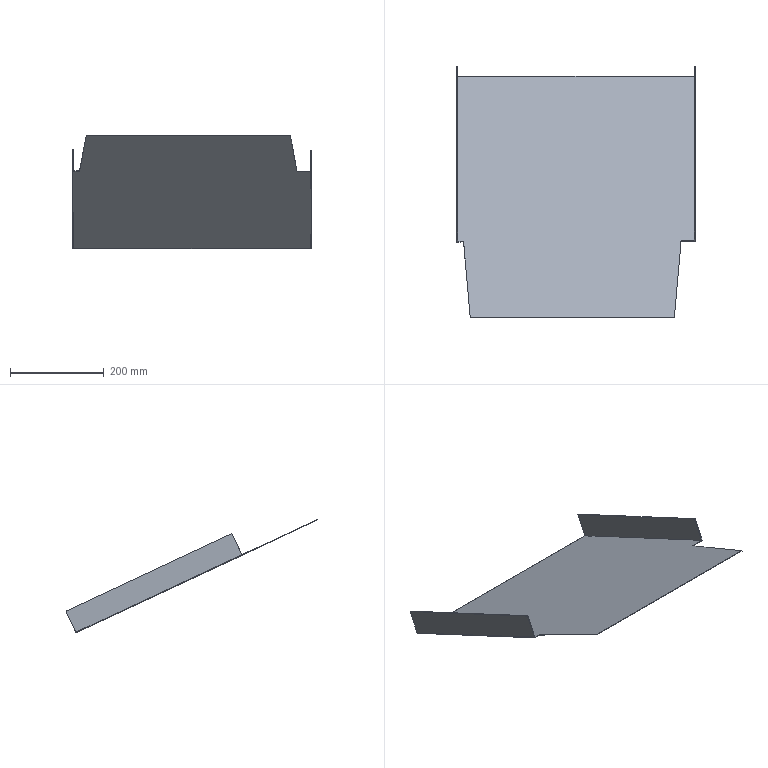Part | NX | features solid 2 | 1 solid | 17 faces | box 510 x 538.761 x 242.084 mm | volume 358465 mm3 | plane 15 | spline 2
STEP:
#1=CARTESIAN_POINT('',(348.,1102.315,-269.141));
#2=VERTEX_POINT('',#1);
#3=CARTESIAN_POINT('',(-158.,1102.315,-269.141));
#4=VERTEX_POINT('',#3);
#5=CARTESIAN_POINT('',(-1100.,1102.315,-269.141));
#6=DIRECTION('',(1.,0.,0.));
#7=VECTOR('',#6,1000.);
#8=LINE('',#5,#7);
#9=EDGE_CURVE('',#2,#4,#8,.F.);
#10=ORIENTED_EDGE('',*,*,#9,.T.);
#11=CARTESIAN_POINT('',(-158.,747.462,-103.67));
#12=VERTEX_POINT('',#11);
#13=CARTESIAN_POINT('',(-158.,630.423,-49.094));
#14=DIRECTION('',(0.,0.9063,-0.4226));
#15=VECTOR('',#14,1000.);
#16=LINE('',#13,#15);
#17=EDGE_CURVE('',#4,#12,#16,.F.);
#18=ORIENTED_EDGE('',*,*,#17,.T.);
#19=CARTESIAN_POINT('',(-145.428,747.563,-103.717));
#20=VERTEX_POINT('',#19);
#21=CARTESIAN_POINT('',(-145.428,747.563,-103.717));
#22=CARTESIAN_POINT('',(-148.187,747.54,-103.707));
#23=CARTESIAN_POINT('',(-152.378,747.509,-103.692));
#24=CARTESIAN_POINT('',(-158.,747.469,-103.673));
#25=B_SPLINE_CURVE_WITH_KNOTS('',3,(#21,#22,#23,#24),.UNSPECIFIED.,.F.,.F.,(4,4),(0.,0.1284),.UNSPECIFIED.);
#26=EDGE_CURVE('',#12,#20,#25,.F.);
#27=ORIENTED_EDGE('',*,*,#26,.T.);
#28=CARTESIAN_POINT('',(-131.215,585.107,-27.963));
#29=VERTEX_POINT('',#28);
#30=CARTESIAN_POINT('',(-37.805,-482.577,469.906));
#31=DIRECTION('',(0.07904,-0.9035,0.4213));
#32=VECTOR('',#31,1000.);
#33=LINE('',#30,#32);
#34=EDGE_CURVE('',#29,#20,#33,.F.);
#35=ORIENTED_EDGE('',*,*,#34,.F.);
#36=CARTESIAN_POINT('',(305.318,585.107,-27.963));
#37=VERTEX_POINT('',#36);
#38=CARTESIAN_POINT('',(-1100.,585.107,-27.963));
#39=DIRECTION('',(-1.,0.,0.));
#40=VECTOR('',#39,1000.);
#41=LINE('',#38,#40);
#42=EDGE_CURVE('',#29,#37,#41,.F.);
#43=ORIENTED_EDGE('',*,*,#42,.T.);
#44=CARTESIAN_POINT('',(319.689,749.371,-104.56));
#45=VERTEX_POINT('',#44);
#46=CARTESIAN_POINT('',(300.478,529.781,-2.164));
#47=DIRECTION('',(0.07904,0.9035,-0.4213));
#48=VECTOR('',#47,1000.);
#49=LINE('',#46,#48);
#50=EDGE_CURVE('',#45,#37,#49,.F.);
#51=ORIENTED_EDGE('',*,*,#50,.F.);
#52=CARTESIAN_POINT('',(348.,749.432,-104.589));
#53=VERTEX_POINT('',#52);
#54=CARTESIAN_POINT('',(348.,749.428,-104.587));
#55=CARTESIAN_POINT('',(338.843,749.394,-104.571));
#56=CARTESIAN_POINT('',(329.406,749.375,-104.562));
#57=CARTESIAN_POINT('',(319.689,749.371,-104.56));
#58=B_SPLINE_CURVE_WITH_KNOTS('',3,(#54,#55,#56,#57),.UNSPECIFIED.,.F.,.F.,(4,4),(0.8994,1.),.UNSPECIFIED.);
#59=EDGE_CURVE('',#53,#45,#58,.T.);
#60=ORIENTED_EDGE('',*,*,#59,.F.);
#61=CARTESIAN_POINT('',(348.,630.423,-49.094));
#62=DIRECTION('',(0.,0.9063,-0.4226));
#63=VECTOR('',#62,1000.);
#64=LINE('',#61,#63);
#65=EDGE_CURVE('',#2,#53,#64,.F.);
#66=ORIENTED_EDGE('',*,*,#65,.F.);
#67=EDGE_LOOP('',(#10,#18,#27,#35,#43,#51,#60,#66));
#68=FACE_BOUND('',#67,.T.);
#69=CARTESIAN_POINT('',(-1100.,630.423,-49.094));
#70=DIRECTION('',(0.,-0.4226,-0.9063));
#71=DIRECTION('',(0.,-0.9063,0.4226));
#72=AXIS2_PLACEMENT_3D('',#69,#70,#71);
#73=PLANE('',#72);
#74=ADVANCED_FACE('',(#68),#73,.F.);
#75=CARTESIAN_POINT('',(350.,1101.892,-270.047));
#76=VERTEX_POINT('',#75);
#77=CARTESIAN_POINT('',(-160.,1101.892,-270.047));
#78=VERTEX_POINT('',#77);
#79=CARTESIAN_POINT('',(-1100.,1101.892,-270.047));
#80=DIRECTION('',(1.,0.,0.));
#81=VECTOR('',#80,1000.);
#82=LINE('',#79,#81);
#83=EDGE_CURVE('',#76,#78,#82,.F.);
#84=ORIENTED_EDGE('',*,*,#83,.F.);
#85=CARTESIAN_POINT('',(350.,749.013,-105.497));
#86=VERTEX_POINT('',#85);
#87=CARTESIAN_POINT('',(350.,630.,-50.));
#88=DIRECTION('',(0.,0.9063,-0.4226));
#89=VECTOR('',#88,1000.);
#90=LINE('',#87,#89);
#91=EDGE_CURVE('',#76,#86,#90,.F.);
#92=ORIENTED_EDGE('',*,*,#91,.T.);
#93=CARTESIAN_POINT('',(319.689,748.949,-105.467));
#94=VERTEX_POINT('',#93);
#95=CARTESIAN_POINT('',(350.,749.013,-105.497));
#96=CARTESIAN_POINT('',(340.219,748.974,-105.478));
#97=CARTESIAN_POINT('',(330.116,748.953,-105.468));
#98=CARTESIAN_POINT('',(319.689,748.949,-105.467));
#99=B_SPLINE_CURVE_WITH_KNOTS('',3,(#95,#96,#97,#98),.UNSPECIFIED.,.F.,.F.,(4,4),(0.8921,1.),.UNSPECIFIED.);
#100=EDGE_CURVE('',#86,#94,#99,.T.);
#101=ORIENTED_EDGE('',*,*,#100,.T.);
#102=CARTESIAN_POINT('',(305.318,584.685,-28.869));
#103=VERTEX_POINT('',#102);
#104=CARTESIAN_POINT('',(300.478,529.358,-3.07));
#105=DIRECTION('',(0.07904,0.9035,-0.4213));
#106=VECTOR('',#105,1000.);
#107=LINE('',#104,#106);
#108=EDGE_CURVE('',#94,#103,#107,.F.);
#109=ORIENTED_EDGE('',*,*,#108,.T.);
#110=CARTESIAN_POINT('',(-131.215,584.685,-28.869));
#111=VERTEX_POINT('',#110);
#112=CARTESIAN_POINT('',(-1100.,584.685,-28.869));
#113=DIRECTION('',(-1.,0.,0.));
#114=VECTOR('',#113,1000.);
#115=LINE('',#112,#114);
#116=EDGE_CURVE('',#111,#103,#115,.F.);
#117=ORIENTED_EDGE('',*,*,#116,.F.);
#118=CARTESIAN_POINT('',(-145.428,747.141,-104.624));
#119=VERTEX_POINT('',#118);
#120=CARTESIAN_POINT('',(-37.805,-482.999,469.));
#121=DIRECTION('',(0.07904,-0.9035,0.4213));
#122=VECTOR('',#121,1000.);
#123=LINE('',#120,#122);
#124=EDGE_CURVE('',#111,#119,#123,.F.);
#125=ORIENTED_EDGE('',*,*,#124,.T.);
#126=CARTESIAN_POINT('',(-158.,747.043,-104.578));
#127=VERTEX_POINT('',#126);
#128=CARTESIAN_POINT('',(-145.428,747.141,-104.624));
#129=CARTESIAN_POINT('',(-148.187,747.118,-104.613));
#130=CARTESIAN_POINT('',(-152.378,747.087,-104.598));
#131=CARTESIAN_POINT('',(-158.,747.047,-104.58));
#132=B_SPLINE_CURVE_WITH_KNOTS('',3,(#128,#129,#130,#131),.UNSPECIFIED.,.F.,.F.,(4,4),(0.,0.1284),.UNSPECIFIED.);
#133=EDGE_CURVE('',#127,#119,#132,.F.);
#134=ORIENTED_EDGE('',*,*,#133,.F.);
#135=CARTESIAN_POINT('',(-160.,747.032,-104.573));
#136=VERTEX_POINT('',#135);
#137=CARTESIAN_POINT('',(-158.,747.047,-104.58));
#138=CARTESIAN_POINT('',(-158.648,747.042,-104.578));
#139=CARTESIAN_POINT('',(-159.314,747.037,-104.575));
#140=CARTESIAN_POINT('',(-160.,747.032,-104.573));
#141=B_SPLINE_CURVE_WITH_KNOTS('',3,(#137,#138,#139,#140),.UNSPECIFIED.,.F.,.F.,(4,4),(0.1284,0.1432),.UNSPECIFIED.);
#142=EDGE_CURVE('',#127,#136,#141,.T.);
#143=ORIENTED_EDGE('',*,*,#142,.T.);
#144=CARTESIAN_POINT('',(-160.,630.,-50.));
#145=DIRECTION('',(0.,0.9063,-0.4226));
#146=VECTOR('',#145,1000.);
#147=LINE('',#144,#146);
#148=EDGE_CURVE('',#78,#136,#147,.F.);
#149=ORIENTED_EDGE('',*,*,#148,.F.);
#150=EDGE_LOOP('',(#84,#92,#101,#109,#117,#125,#134,#143,#149));
#151=FACE_BOUND('',#150,.T.);
#152=CARTESIAN_POINT('',(-1100.,630.,-50.));
#153=DIRECTION('',(0.,-0.4226,-0.9063));
#154=DIRECTION('',(0.,-0.9063,0.4226));
#155=AXIS2_PLACEMENT_3D('',#152,#153,#154);
#156=PLANE('',#155);
#157=ADVANCED_FACE('',(#151),#156,.T.);
#158=CARTESIAN_POINT('',(350.,1123.446,-223.825));
#159=VERTEX_POINT('',#158);
#160=CARTESIAN_POINT('',(350.,1101.892,-270.047));
#161=DIRECTION('',(0.,-0.4226,-0.9063));
#162=VECTOR('',#161,1000.);
#163=LINE('',#160,#162);
#164=EDGE_CURVE('',#159,#76,#163,.T.);
#165=ORIENTED_EDGE('',*,*,#164,.T.);
#166=ORIENTED_EDGE('',*,*,#83,.T.);
#167=CARTESIAN_POINT('',(-160.,1123.446,-223.825));
#168=VERTEX_POINT('',#167);
#169=CARTESIAN_POINT('',(-160.,1101.892,-270.047));
#170=DIRECTION('',(0.,-0.4226,-0.9063));
#171=VECTOR('',#170,1000.);
#172=LINE('',#169,#171);
#173=EDGE_CURVE('',#168,#78,#172,.T.);
#174=ORIENTED_EDGE('',*,*,#173,.F.);
#175=CARTESIAN_POINT('',(-158.,1123.446,-223.825));
#176=VERTEX_POINT('',#175);
#177=CARTESIAN_POINT('',(-160.,1123.446,-223.825));
#178=DIRECTION('',(1.,0.,0.));
#179=VECTOR('',#178,1000.);
#180=LINE('',#177,#179);
#181=EDGE_CURVE('',#176,#168,#180,.F.);
#182=ORIENTED_EDGE('',*,*,#181,.F.);
#183=CARTESIAN_POINT('',(-158.,1101.892,-270.047));
#184=DIRECTION('',(0.,0.4226,0.9063));
#185=VECTOR('',#184,1000.);
#186=LINE('',#183,#185);
#187=EDGE_CURVE('',#4,#176,#186,.T.);
#188=ORIENTED_EDGE('',*,*,#187,.F.);
#189=ORIENTED_EDGE('',*,*,#9,.F.);
#190=CARTESIAN_POINT('',(348.,1123.446,-223.825));
#191=VERTEX_POINT('',#190);
#192=CARTESIAN_POINT('',(348.,1101.892,-270.047));
#193=DIRECTION('',(0.,0.4226,0.9063));
#194=VECTOR('',#193,1000.);
#195=LINE('',#192,#194);
#196=EDGE_CURVE('',#2,#191,#195,.T.);
#197=ORIENTED_EDGE('',*,*,#196,.T.);
#198=CARTESIAN_POINT('',(350.,1123.446,-223.825));
#199=DIRECTION('',(1.,0.,0.));
#200=VECTOR('',#199,1000.);
#201=LINE('',#198,#200);
#202=EDGE_CURVE('',#191,#159,#201,.T.);
#203=ORIENTED_EDGE('',*,*,#202,.T.);
#204=EDGE_LOOP('',(#165,#166,#174,#182,#188,#189,#197,#203));
#205=FACE_BOUND('',#204,.T.);
#206=CARTESIAN_POINT('',(-1100.,1101.892,-270.047));
#207=DIRECTION('',(0.,-0.9063,0.4226));
#208=DIRECTION('',(0.,0.4226,0.9063));
#209=AXIS2_PLACEMENT_3D('',#206,#207,#208);
#210=PLANE('',#209);
#211=ADVANCED_FACE('',(#205),#210,.F.);
#212=CARTESIAN_POINT('',(350.,749.436,-104.59));
#213=VERTEX_POINT('',#212);
#214=CARTESIAN_POINT('',(350.,749.436,-104.59));
#215=CARTESIAN_POINT('',(349.333,749.436,-104.59));
#216=CARTESIAN_POINT('',(348.667,749.436,-104.59));
#217=CARTESIAN_POINT('',(348.,749.436,-104.59));
#218=B_SPLINE_CURVE_WITH_KNOTS('',3,(#214,#215,#216,#217),.UNSPECIFIED.,.F.,.F.,(4,4),(0.,1.),.UNSPECIFIED.);
#219=EDGE_CURVE('',#213,#53,#218,.T.);
#220=ORIENTED_EDGE('',*,*,#219,.T.);
#221=ORIENTED_EDGE('',*,*,#59,.T.);
#222=CARTESIAN_POINT('',(319.689,748.949,-105.467));
#223=CARTESIAN_POINT('',(319.689,749.09,-105.165));
#224=CARTESIAN_POINT('',(319.689,749.23,-104.862));
#225=CARTESIAN_POINT('',(319.689,749.371,-104.56));
#226=B_SPLINE_CURVE_WITH_KNOTS('',3,(#222,#223,#224,#225),.UNSPECIFIED.,.F.,.F.,(4,4),(0.,1.),.UNSPECIFIED.);
#227=EDGE_CURVE('',#94,#45,#226,.T.);
#228=ORIENTED_EDGE('',*,*,#227,.F.);
#229=ORIENTED_EDGE('',*,*,#100,.F.);
#230=CARTESIAN_POINT('',(350.,749.013,-105.497));
#231=DIRECTION('',(0.,0.4226,0.9063));
#232=VECTOR('',#231,1000.);
#233=LINE('',#230,#232);
#234=EDGE_CURVE('',#213,#86,#233,.F.);
#235=ORIENTED_EDGE('',*,*,#234,.F.);
#236=EDGE_LOOP('',(#220,#221,#228,#229,#235));
#237=FACE_BOUND('',#236,.T.);
#238=CARTESIAN_POINT('',(350.,749.013,-105.497));
#239=CARTESIAN_POINT('',(350.,749.436,-104.59));
#240=CARTESIAN_POINT('',(340.219,748.974,-105.478));
#241=CARTESIAN_POINT('',(340.219,749.397,-104.572));
#242=CARTESIAN_POINT('',(330.116,748.953,-105.468));
#243=CARTESIAN_POINT('',(330.116,749.375,-104.562));
#244=CARTESIAN_POINT('',(319.689,748.949,-105.467));
#245=CARTESIAN_POINT('',(319.689,749.371,-104.56));
#246=B_SPLINE_SURFACE_WITH_KNOTS('',3,1,((#238,#239),(#240,#241),(#242,#243),(#244,#245)),.SURF_OF_LINEAR_EXTRUSION.,.F.,.F.,.F.,(4,4),(2,2),(0.8921,1.),(0.,1.),.PIECEWISE_BEZIER_KNOTS.);
#247=ADVANCED_FACE('',(#237),#246,.F.);
#248=ORIENTED_EDGE('',*,*,#133,.T.);
#249=CARTESIAN_POINT('',(-145.428,747.563,-103.717));
#250=CARTESIAN_POINT('',(-145.428,747.422,-104.019));
#251=CARTESIAN_POINT('',(-145.428,747.281,-104.321));
#252=CARTESIAN_POINT('',(-145.428,747.141,-104.624));
#253=B_SPLINE_CURVE_WITH_KNOTS('',3,(#249,#250,#251,#252),.UNSPECIFIED.,.F.,.F.,(4,4),(0.,1.),.UNSPECIFIED.);
#254=EDGE_CURVE('',#119,#20,#253,.F.);
#255=ORIENTED_EDGE('',*,*,#254,.T.);
#256=ORIENTED_EDGE('',*,*,#26,.F.);
#257=CARTESIAN_POINT('',(-158.,747.047,-104.58));
#258=DIRECTION('',(0.,0.4226,0.9063));
#259=VECTOR('',#258,1000.);
#260=LINE('',#257,#259);
#261=EDGE_CURVE('',#127,#12,#260,.T.);
#262=ORIENTED_EDGE('',*,*,#261,.F.);
#263=EDGE_LOOP('',(#248,#255,#256,#262));
#264=FACE_BOUND('',#263,.T.);
#265=CARTESIAN_POINT('',(-145.428,747.141,-104.624));
#266=CARTESIAN_POINT('',(-145.428,747.563,-103.717));
#267=CARTESIAN_POINT('',(-148.204,747.118,-104.613));
#268=CARTESIAN_POINT('',(-148.204,747.54,-103.707));
#269=CARTESIAN_POINT('',(-152.428,747.086,-104.598));
#270=CARTESIAN_POINT('',(-152.428,747.509,-103.692));
#271=CARTESIAN_POINT('',(-158.101,747.046,-104.579));
#272=CARTESIAN_POINT('',(-158.101,747.469,-103.673));
#273=B_SPLINE_SURFACE_WITH_KNOTS('',3,1,((#265,#266),(#267,#268),(#269,#270),(#271,#272)),.SURF_OF_LINEAR_EXTRUSION.,.F.,.F.,.F.,(4,4),(2,2),(0.,0.1292),(0.,1.),.PIECEWISE_BEZIER_KNOTS.);
#274=ADVANCED_FACE('',(#264),#273,.F.);
#275=ORIENTED_EDGE('',*,*,#34,.T.);
#276=ORIENTED_EDGE('',*,*,#254,.F.);
#277=ORIENTED_EDGE('',*,*,#124,.F.);
#278=CARTESIAN_POINT('',(-131.215,584.685,-28.869));
#279=DIRECTION('',(0.,0.4226,0.9063));
#280=VECTOR('',#279,1000.);
#281=LINE('',#278,#280);
#282=EDGE_CURVE('',#111,#29,#281,.T.);
#283=ORIENTED_EDGE('',*,*,#282,.T.);
#284=EDGE_LOOP('',(#275,#276,#277,#283));
#285=FACE_BOUND('',#284,.T.);
#286=CARTESIAN_POINT('',(-37.805,-482.999,469.));
#287=DIRECTION('',(-0.9969,-0.07164,0.03341));
#288=DIRECTION('',(-0.07168,0.9974,0.));
#289=AXIS2_PLACEMENT_3D('',#286,#287,#288);
#290=PLANE('',#289);
#291=ADVANCED_FACE('',(#285),#290,.T.);
#292=ORIENTED_EDGE('',*,*,#42,.F.);
#293=ORIENTED_EDGE('',*,*,#282,.F.);
#294=ORIENTED_EDGE('',*,*,#116,.T.);
#295=CARTESIAN_POINT('',(305.318,584.685,-28.869));
#296=DIRECTION('',(0.,0.4226,0.9063));
#297=VECTOR('',#296,1000.);
#298=LINE('',#295,#297);
#299=EDGE_CURVE('',#103,#37,#298,.T.);
#300=ORIENTED_EDGE('',*,*,#299,.T.);
#301=EDGE_LOOP('',(#292,#293,#294,#300));
#302=FACE_BOUND('',#301,.T.);
#303=CARTESIAN_POINT('',(-1100.,584.685,-28.869));
#304=DIRECTION('',(0.,0.9063,-0.4226));
#305=DIRECTION('',(0.,-0.4226,-0.9063));
#306=AXIS2_PLACEMENT_3D('',#303,#304,#305);
#307=PLANE('',#306);
#308=ADVANCED_FACE('',(#302),#307,.F.);
#309=ORIENTED_EDGE('',*,*,#50,.T.);
#310=ORIENTED_EDGE('',*,*,#299,.F.);
#311=ORIENTED_EDGE('',*,*,#108,.F.);
#312=ORIENTED_EDGE('',*,*,#227,.T.);
#313=EDGE_LOOP('',(#309,#310,#311,#312));
#314=FACE_BOUND('',#313,.T.);
#315=CARTESIAN_POINT('',(300.478,529.358,-3.07));
#316=DIRECTION('',(0.9969,-0.07164,0.03341));
#317=DIRECTION('',(-0.07168,-0.9974,0.));
#318=AXIS2_PLACEMENT_3D('',#315,#316,#317);
#319=PLANE('',#318);
#320=ADVANCED_FACE('',(#314),#319,.T.);
#321=ORIENTED_EDGE('',*,*,#234,.T.);
#322=ORIENTED_EDGE('',*,*,#91,.F.);
#323=ORIENTED_EDGE('',*,*,#164,.F.);
#324=CARTESIAN_POINT('',(350.,770.567,-59.275));
#325=VERTEX_POINT('',#324);
#326=CARTESIAN_POINT('',(350.,1123.446,-223.825));
#327=DIRECTION('',(0.,-0.9063,0.4226));
#328=VECTOR('',#327,1000.);
#329=LINE('',#326,#328);
#330=EDGE_CURVE('',#159,#325,#329,.T.);
#331=ORIENTED_EDGE('',*,*,#330,.T.);
#332=CARTESIAN_POINT('',(350.,749.013,-105.497));
#333=DIRECTION('',(0.,0.4226,0.9063));
#334=VECTOR('',#333,1000.);
#335=LINE('',#332,#334);
#336=EDGE_CURVE('',#213,#325,#335,.T.);
#337=ORIENTED_EDGE('',*,*,#336,.F.);
#338=EDGE_LOOP('',(#321,#322,#323,#331,#337));
#339=FACE_BOUND('',#338,.T.);
#340=CARTESIAN_POINT('',(350.,0.,0.));
#341=DIRECTION('',(1.,0.,0.));
#342=DIRECTION('',(0.,0.,-1.));
#343=AXIS2_PLACEMENT_3D('',#340,#341,#342);
#344=PLANE('',#343);
#345=ADVANCED_FACE('',(#339),#344,.T.);
#346=ORIENTED_EDGE('',*,*,#173,.T.);
#347=ORIENTED_EDGE('',*,*,#148,.T.);
#348=CARTESIAN_POINT('',(-160.,768.586,-58.351));
#349=VERTEX_POINT('',#348);
#350=CARTESIAN_POINT('',(-160.,747.032,-104.573));
#351=DIRECTION('',(0.,0.4226,0.9063));
#352=VECTOR('',#351,1000.);
#353=LINE('',#350,#352);
#354=EDGE_CURVE('',#136,#349,#353,.T.);
#355=ORIENTED_EDGE('',*,*,#354,.T.);
#356=CARTESIAN_POINT('',(-160.,1123.446,-223.825));
#357=DIRECTION('',(0.,-0.9063,0.4226));
#358=VECTOR('',#357,1000.);
#359=LINE('',#356,#358);
#360=EDGE_CURVE('',#168,#349,#359,.T.);
#361=ORIENTED_EDGE('',*,*,#360,.F.);
#362=EDGE_LOOP('',(#346,#347,#355,#361));
#363=FACE_BOUND('',#362,.T.);
#364=CARTESIAN_POINT('',(-160.,0.,0.));
#365=DIRECTION('',(1.,0.,0.));
#366=DIRECTION('',(0.,0.,-1.));
#367=AXIS2_PLACEMENT_3D('',#364,#365,#366);
#368=PLANE('',#367);
#369=ADVANCED_FACE('',(#363),#368,.F.);
#370=ORIENTED_EDGE('',*,*,#261,.T.);
#371=CARTESIAN_POINT('',(-158.,747.032,-104.573));
#372=DIRECTION('',(0.,0.4226,0.9063));
#373=VECTOR('',#372,1000.);
#374=LINE('',#371,#373);
#375=EDGE_CURVE('',#127,#12,#374,.T.);
#376=ORIENTED_EDGE('',*,*,#375,.F.);
#377=EDGE_LOOP('',(#370,#376));
#378=FACE_BOUND('',#377,.T.);
#379=CARTESIAN_POINT('',(-158.,1101.892,-270.047));
#380=DIRECTION('',(1.,0.,0.));
#381=DIRECTION('',(0.,0.,-1.));
#382=AXIS2_PLACEMENT_3D('',#379,#380,#381);
#383=PLANE('',#382);
#384=ADVANCED_FACE('',(#378),#383,.T.);
#385=ORIENTED_EDGE('',*,*,#354,.F.);
#386=ORIENTED_EDGE('',*,*,#142,.F.);
#387=ORIENTED_EDGE('',*,*,#375,.T.);
#388=CARTESIAN_POINT('',(-158.,768.586,-58.351));
#389=VERTEX_POINT('',#388);
#390=CARTESIAN_POINT('',(-158.,747.032,-104.573));
#391=DIRECTION('',(0.,0.4226,0.9063));
#392=VECTOR('',#391,1000.);
#393=LINE('',#390,#392);
#394=EDGE_CURVE('',#12,#389,#393,.T.);
#395=ORIENTED_EDGE('',*,*,#394,.T.);
#396=CARTESIAN_POINT('',(-160.,768.586,-58.351));
#397=DIRECTION('',(1.,0.,0.));
#398=VECTOR('',#397,1000.);
#399=LINE('',#396,#398);
#400=EDGE_CURVE('',#389,#349,#399,.F.);
#401=ORIENTED_EDGE('',*,*,#400,.T.);
#402=EDGE_LOOP('',(#385,#386,#387,#395,#401));
#403=FACE_BOUND('',#402,.T.);
#404=CARTESIAN_POINT('',(-160.,747.032,-104.573));
#405=DIRECTION('',(0.,-0.9063,0.4226));
#406=DIRECTION('',(0.,0.4226,0.9063));
#407=AXIS2_PLACEMENT_3D('',#404,#405,#406);
#408=PLANE('',#407);
#409=ADVANCED_FACE('',(#403),#408,.T.);
#410=ORIENTED_EDGE('',*,*,#400,.F.);
#411=CARTESIAN_POINT('',(-158.,1123.446,-223.825));
#412=DIRECTION('',(0.,-0.9063,0.4226));
#413=VECTOR('',#412,1000.);
#414=LINE('',#411,#413);
#415=EDGE_CURVE('',#176,#389,#414,.T.);
#416=ORIENTED_EDGE('',*,*,#415,.F.);
#417=ORIENTED_EDGE('',*,*,#181,.T.);
#418=ORIENTED_EDGE('',*,*,#360,.T.);
#419=EDGE_LOOP('',(#410,#416,#417,#418));
#420=FACE_BOUND('',#419,.T.);
#421=CARTESIAN_POINT('',(-160.,1123.446,-223.825));
#422=DIRECTION('',(0.,-0.4226,-0.9063));
#423=DIRECTION('',(0.,-0.9063,0.4226));
#424=AXIS2_PLACEMENT_3D('',#421,#422,#423);
#425=PLANE('',#424);
#426=ADVANCED_FACE('',(#420),#425,.F.);
#427=ORIENTED_EDGE('',*,*,#187,.T.);
#428=ORIENTED_EDGE('',*,*,#415,.T.);
#429=ORIENTED_EDGE('',*,*,#394,.F.);
#430=ORIENTED_EDGE('',*,*,#17,.F.);
#431=EDGE_LOOP('',(#427,#428,#429,#430));
#432=FACE_BOUND('',#431,.T.);
#433=CARTESIAN_POINT('',(-158.,1101.892,-270.047));
#434=DIRECTION('',(1.,0.,0.));
#435=DIRECTION('',(0.,0.,-1.));
#436=AXIS2_PLACEMENT_3D('',#433,#434,#435);
#437=PLANE('',#436);
#438=ADVANCED_FACE('',(#432),#437,.T.);
#439=ORIENTED_EDGE('',*,*,#336,.T.);
#440=CARTESIAN_POINT('',(348.,770.567,-59.275));
#441=VERTEX_POINT('',#440);
#442=CARTESIAN_POINT('',(350.,770.567,-59.275));
#443=DIRECTION('',(1.,0.,0.));
#444=VECTOR('',#443,1000.);
#445=LINE('',#442,#444);
#446=EDGE_CURVE('',#441,#325,#445,.T.);
#447=ORIENTED_EDGE('',*,*,#446,.F.);
#448=CARTESIAN_POINT('',(348.,749.013,-105.497));
#449=DIRECTION('',(0.,0.4226,0.9063));
#450=VECTOR('',#449,1000.);
#451=LINE('',#448,#450);
#452=EDGE_CURVE('',#53,#441,#451,.T.);
#453=ORIENTED_EDGE('',*,*,#452,.F.);
#454=ORIENTED_EDGE('',*,*,#219,.F.);
#455=EDGE_LOOP('',(#439,#447,#453,#454));
#456=FACE_BOUND('',#455,.T.);
#457=CARTESIAN_POINT('',(350.,749.013,-105.497));
#458=DIRECTION('',(0.,-0.9063,0.4226));
#459=DIRECTION('',(0.,0.4226,0.9063));
#460=AXIS2_PLACEMENT_3D('',#457,#458,#459);
#461=PLANE('',#460);
#462=ADVANCED_FACE('',(#456),#461,.T.);
#463=ORIENTED_EDGE('',*,*,#446,.T.);
#464=ORIENTED_EDGE('',*,*,#330,.F.);
#465=ORIENTED_EDGE('',*,*,#202,.F.);
#466=CARTESIAN_POINT('',(348.,1123.446,-223.825));
#467=DIRECTION('',(0.,-0.9063,0.4226));
#468=VECTOR('',#467,1000.);
#469=LINE('',#466,#468);
#470=EDGE_CURVE('',#191,#441,#469,.T.);
#471=ORIENTED_EDGE('',*,*,#470,.T.);
#472=EDGE_LOOP('',(#463,#464,#465,#471));
#473=FACE_BOUND('',#472,.T.);
#474=CARTESIAN_POINT('',(350.,1123.446,-223.825));
#475=DIRECTION('',(0.,-0.4226,-0.9063));
#476=DIRECTION('',(0.,-0.9063,0.4226));
#477=AXIS2_PLACEMENT_3D('',#474,#475,#476);
#478=PLANE('',#477);
#479=ADVANCED_FACE('',(#473),#478,.F.);
#480=ORIENTED_EDGE('',*,*,#65,.T.);
#481=ORIENTED_EDGE('',*,*,#452,.T.);
#482=ORIENTED_EDGE('',*,*,#470,.F.);
#483=ORIENTED_EDGE('',*,*,#196,.F.);
#484=EDGE_LOOP('',(#480,#481,#482,#483));
#485=FACE_BOUND('',#484,.T.);
#486=CARTESIAN_POINT('',(348.,1101.892,-270.047));
#487=DIRECTION('',(1.,0.,0.));
#488=DIRECTION('',(0.,0.,-1.));
#489=AXIS2_PLACEMENT_3D('',#486,#487,#488);
#490=PLANE('',#489);
#491=ADVANCED_FACE('',(#485),#490,.F.);
#492=CLOSED_SHELL('',(#74,#157,#211,#247,#274,#291,#308,#320,#345,#369,#384,#409,#426,#438,#462,#479,#491));
#493=MANIFOLD_SOLID_BREP('',#492);
#494=(LENGTH_UNIT()NAMED_UNIT(*)SI_UNIT(.MILLI.,.METRE.));
#495=UNCERTAINTY_MEASURE_WITH_UNIT(LENGTH_MEASURE(0.07428),#494,'','');
#496=(NAMED_UNIT(*)PLANE_ANGLE_UNIT()SI_UNIT($,.RADIAN.));
#497=(NAMED_UNIT(*)SI_UNIT($,.STERADIAN.)SOLID_ANGLE_UNIT());
#498=(GEOMETRIC_REPRESENTATION_CONTEXT(3)GLOBAL_UNCERTAINTY_ASSIGNED_CONTEXT((#495))GLOBAL_UNIT_ASSIGNED_CONTEXT((#494,#496,#497))REPRESENTATION_CONTEXT('',''));
#499=ADVANCED_BREP_SHAPE_REPRESENTATION('',(#493),#498);